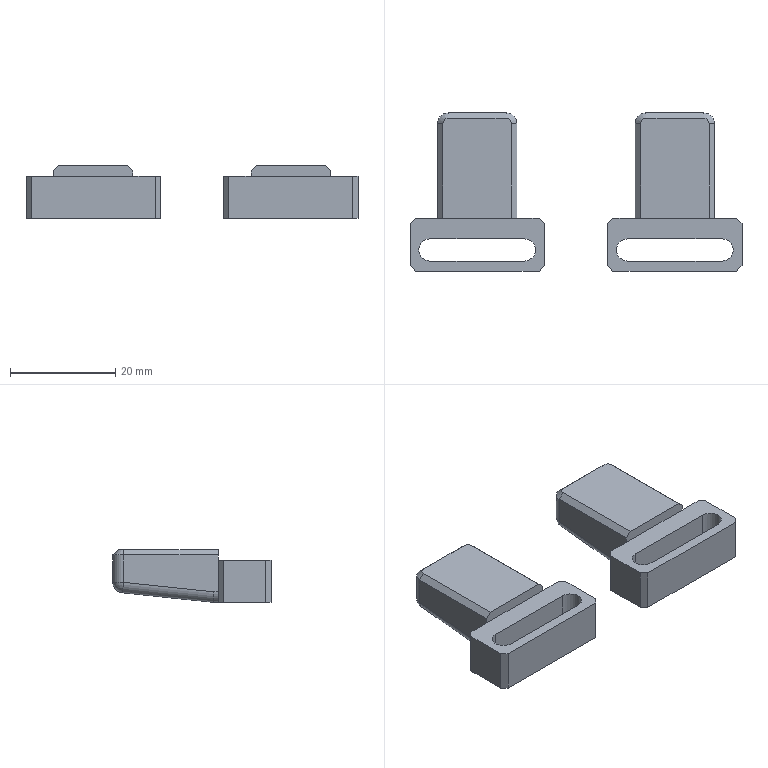Part | 2 solids | 78 faces | box 63 x 30 x 10 mm | volume 7074 mm3 | plane 48 | cylinder 22 | sphere 4 | cone 4 | commonest cylinder face diameters 4 x16 4.2 x4 10 x2